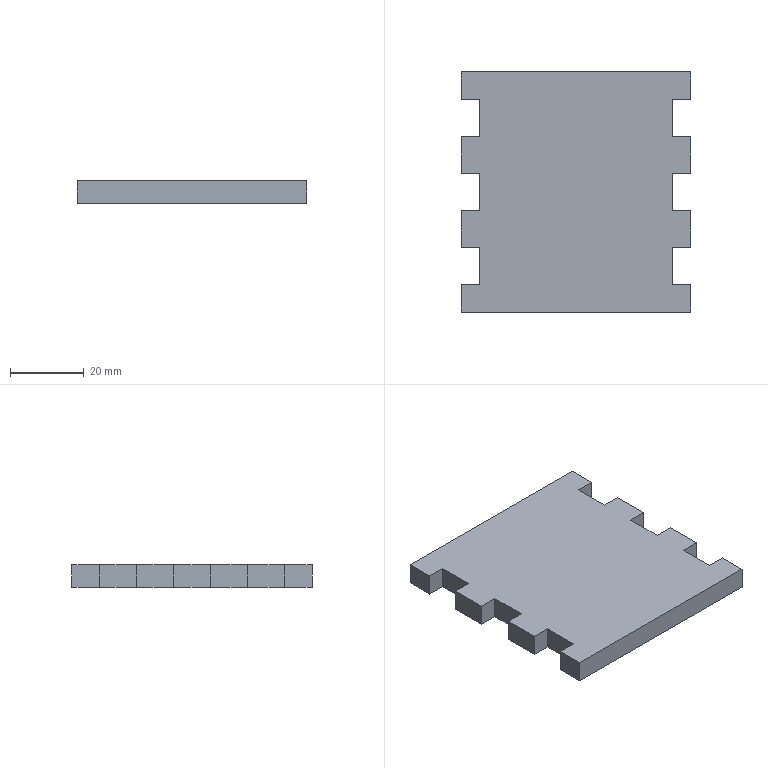Part | SolidWorks | features FlatPattern 1, SMBaseFlange 1, SheetMetal 1 | 1 solid | 30 faces | box 62 x 65 x 6 mm | volume 22380 mm3 | plane 30
STEP:
#1=CARTESIAN_POINT('',(31.,57.5,0.));
#2=VERTEX_POINT('',#1);
#3=CARTESIAN_POINT('',(31.,65.,0.));
#4=VERTEX_POINT('',#3);
#5=CARTESIAN_POINT('',(31.,65.,0.));
#6=DIRECTION('',(0.,1.,0.));
#7=VECTOR('',#6,1000.);
#8=LINE('',#5,#7);
#9=EDGE_CURVE('',#2,#4,#8,.T.);
#10=ORIENTED_EDGE('',*,*,#9,.T.);
#11=CARTESIAN_POINT('',(31.,65.,6.));
#12=VERTEX_POINT('',#11);
#13=CARTESIAN_POINT('',(31.,65.,6.));
#14=DIRECTION('',(0.,0.,-1.));
#15=VECTOR('',#14,1000.);
#16=LINE('',#13,#15);
#17=EDGE_CURVE('',#12,#4,#16,.T.);
#18=ORIENTED_EDGE('',*,*,#17,.F.);
#19=CARTESIAN_POINT('',(31.,57.5,6.));
#20=VERTEX_POINT('',#19);
#21=CARTESIAN_POINT('',(31.,65.,6.));
#22=DIRECTION('',(0.,1.,0.));
#23=VECTOR('',#22,1000.);
#24=LINE('',#21,#23);
#25=EDGE_CURVE('',#20,#12,#24,.T.);
#26=ORIENTED_EDGE('',*,*,#25,.F.);
#27=CARTESIAN_POINT('',(31.,57.5,6.));
#28=DIRECTION('',(0.,0.,-1.));
#29=VECTOR('',#28,1000.);
#30=LINE('',#27,#29);
#31=EDGE_CURVE('',#20,#2,#30,.T.);
#32=ORIENTED_EDGE('',*,*,#31,.T.);
#33=EDGE_LOOP('',(#10,#18,#26,#32));
#34=FACE_OUTER_BOUND('',#33,.T.);
#35=CARTESIAN_POINT('',(31.,65.,6.));
#36=DIRECTION('',(-1.,0.,0.));
#37=DIRECTION('',(0.,-1.,0.));
#38=AXIS2_PLACEMENT_3D('',#35,#36,#37);
#39=PLANE('',#38);
#40=ADVANCED_FACE('',(#34),#39,.F.);
#41=CARTESIAN_POINT('',(-31.,65.,0.));
#42=VERTEX_POINT('',#41);
#43=CARTESIAN_POINT('',(31.,65.,0.));
#44=DIRECTION('',(-1.,0.,0.));
#45=VECTOR('',#44,1000.);
#46=LINE('',#43,#45);
#47=EDGE_CURVE('',#4,#42,#46,.T.);
#48=ORIENTED_EDGE('',*,*,#47,.T.);
#49=CARTESIAN_POINT('',(-31.,65.,6.));
#50=VERTEX_POINT('',#49);
#51=CARTESIAN_POINT('',(-31.,65.,6.));
#52=DIRECTION('',(0.,0.,-1.));
#53=VECTOR('',#52,1000.);
#54=LINE('',#51,#53);
#55=EDGE_CURVE('',#50,#42,#54,.T.);
#56=ORIENTED_EDGE('',*,*,#55,.F.);
#57=CARTESIAN_POINT('',(31.,65.,6.));
#58=DIRECTION('',(-1.,0.,0.));
#59=VECTOR('',#58,1000.);
#60=LINE('',#57,#59);
#61=EDGE_CURVE('',#12,#50,#60,.T.);
#62=ORIENTED_EDGE('',*,*,#61,.F.);
#63=ORIENTED_EDGE('',*,*,#17,.T.);
#64=EDGE_LOOP('',(#48,#56,#62,#63));
#65=FACE_OUTER_BOUND('',#64,.T.);
#66=CARTESIAN_POINT('',(31.,65.,6.));
#67=DIRECTION('',(0.,-1.,0.));
#68=DIRECTION('',(1.,0.,0.));
#69=AXIS2_PLACEMENT_3D('',#66,#67,#68);
#70=PLANE('',#69);
#71=ADVANCED_FACE('',(#65),#70,.F.);
#72=CARTESIAN_POINT('',(-31.,57.5,0.));
#73=VERTEX_POINT('',#72);
#74=CARTESIAN_POINT('',(-31.,65.,0.));
#75=DIRECTION('',(0.,-1.,0.));
#76=VECTOR('',#75,1000.);
#77=LINE('',#74,#76);
#78=EDGE_CURVE('',#42,#73,#77,.T.);
#79=ORIENTED_EDGE('',*,*,#78,.T.);
#80=CARTESIAN_POINT('',(-31.,57.5,6.));
#81=VERTEX_POINT('',#80);
#82=CARTESIAN_POINT('',(-31.,57.5,6.));
#83=DIRECTION('',(0.,0.,-1.));
#84=VECTOR('',#83,1000.);
#85=LINE('',#82,#84);
#86=EDGE_CURVE('',#81,#73,#85,.T.);
#87=ORIENTED_EDGE('',*,*,#86,.F.);
#88=CARTESIAN_POINT('',(-31.,65.,6.));
#89=DIRECTION('',(0.,-1.,0.));
#90=VECTOR('',#89,1000.);
#91=LINE('',#88,#90);
#92=EDGE_CURVE('',#50,#81,#91,.T.);
#93=ORIENTED_EDGE('',*,*,#92,.F.);
#94=ORIENTED_EDGE('',*,*,#55,.T.);
#95=EDGE_LOOP('',(#79,#87,#93,#94));
#96=FACE_OUTER_BOUND('',#95,.T.);
#97=CARTESIAN_POINT('',(-31.,65.,6.));
#98=DIRECTION('',(1.,0.,0.));
#99=DIRECTION('',(0.,1.,0.));
#100=AXIS2_PLACEMENT_3D('',#97,#98,#99);
#101=PLANE('',#100);
#102=ADVANCED_FACE('',(#96),#101,.F.);
#103=CARTESIAN_POINT('',(-26.,57.5,0.));
#104=VERTEX_POINT('',#103);
#105=CARTESIAN_POINT('',(-31.,57.5,0.));
#106=DIRECTION('',(1.,0.,0.));
#107=VECTOR('',#106,1000.);
#108=LINE('',#105,#107);
#109=EDGE_CURVE('',#73,#104,#108,.T.);
#110=ORIENTED_EDGE('',*,*,#109,.T.);
#111=CARTESIAN_POINT('',(-26.,57.5,6.));
#112=VERTEX_POINT('',#111);
#113=CARTESIAN_POINT('',(-26.,57.5,6.));
#114=DIRECTION('',(0.,0.,-1.));
#115=VECTOR('',#114,1000.);
#116=LINE('',#113,#115);
#117=EDGE_CURVE('',#112,#104,#116,.T.);
#118=ORIENTED_EDGE('',*,*,#117,.F.);
#119=CARTESIAN_POINT('',(-31.,57.5,6.));
#120=DIRECTION('',(1.,0.,0.));
#121=VECTOR('',#120,1000.);
#122=LINE('',#119,#121);
#123=EDGE_CURVE('',#81,#112,#122,.T.);
#124=ORIENTED_EDGE('',*,*,#123,.F.);
#125=ORIENTED_EDGE('',*,*,#86,.T.);
#126=EDGE_LOOP('',(#110,#118,#124,#125));
#127=FACE_OUTER_BOUND('',#126,.T.);
#128=CARTESIAN_POINT('',(-31.,57.5,6.));
#129=DIRECTION('',(0.,1.,0.));
#130=DIRECTION('',(0.,0.,1.));
#131=AXIS2_PLACEMENT_3D('',#128,#129,#130);
#132=PLANE('',#131);
#133=ADVANCED_FACE('',(#127),#132,.F.);
#134=CARTESIAN_POINT('',(-26.,47.5,0.));
#135=VERTEX_POINT('',#134);
#136=CARTESIAN_POINT('',(-26.,57.5,0.));
#137=DIRECTION('',(0.,-1.,0.));
#138=VECTOR('',#137,1000.);
#139=LINE('',#136,#138);
#140=EDGE_CURVE('',#104,#135,#139,.T.);
#141=ORIENTED_EDGE('',*,*,#140,.T.);
#142=CARTESIAN_POINT('',(-26.,47.5,6.));
#143=VERTEX_POINT('',#142);
#144=CARTESIAN_POINT('',(-26.,47.5,6.));
#145=DIRECTION('',(0.,0.,-1.));
#146=VECTOR('',#145,1000.);
#147=LINE('',#144,#146);
#148=EDGE_CURVE('',#143,#135,#147,.T.);
#149=ORIENTED_EDGE('',*,*,#148,.F.);
#150=CARTESIAN_POINT('',(-26.,57.5,6.));
#151=DIRECTION('',(0.,-1.,0.));
#152=VECTOR('',#151,1000.);
#153=LINE('',#150,#152);
#154=EDGE_CURVE('',#112,#143,#153,.T.);
#155=ORIENTED_EDGE('',*,*,#154,.F.);
#156=ORIENTED_EDGE('',*,*,#117,.T.);
#157=EDGE_LOOP('',(#141,#149,#155,#156));
#158=FACE_OUTER_BOUND('',#157,.T.);
#159=CARTESIAN_POINT('',(-26.,57.5,6.));
#160=DIRECTION('',(1.,0.,0.));
#161=DIRECTION('',(0.,0.,-1.));
#162=AXIS2_PLACEMENT_3D('',#159,#160,#161);
#163=PLANE('',#162);
#164=ADVANCED_FACE('',(#158),#163,.F.);
#165=CARTESIAN_POINT('',(-31.,47.5,0.));
#166=VERTEX_POINT('',#165);
#167=CARTESIAN_POINT('',(-26.,47.5,0.));
#168=DIRECTION('',(-1.,0.,0.));
#169=VECTOR('',#168,1000.);
#170=LINE('',#167,#169);
#171=EDGE_CURVE('',#135,#166,#170,.T.);
#172=ORIENTED_EDGE('',*,*,#171,.T.);
#173=CARTESIAN_POINT('',(-31.,47.5,6.));
#174=VERTEX_POINT('',#173);
#175=CARTESIAN_POINT('',(-31.,47.5,6.));
#176=DIRECTION('',(0.,0.,-1.));
#177=VECTOR('',#176,1000.);
#178=LINE('',#175,#177);
#179=EDGE_CURVE('',#174,#166,#178,.T.);
#180=ORIENTED_EDGE('',*,*,#179,.F.);
#181=CARTESIAN_POINT('',(-26.,47.5,6.));
#182=DIRECTION('',(-1.,0.,0.));
#183=VECTOR('',#182,1000.);
#184=LINE('',#181,#183);
#185=EDGE_CURVE('',#143,#174,#184,.T.);
#186=ORIENTED_EDGE('',*,*,#185,.F.);
#187=ORIENTED_EDGE('',*,*,#148,.T.);
#188=EDGE_LOOP('',(#172,#180,#186,#187));
#189=FACE_OUTER_BOUND('',#188,.T.);
#190=CARTESIAN_POINT('',(-26.,47.5,6.));
#191=DIRECTION('',(0.,-1.,0.));
#192=DIRECTION('',(0.,0.,-1.));
#193=AXIS2_PLACEMENT_3D('',#190,#191,#192);
#194=PLANE('',#193);
#195=ADVANCED_FACE('',(#189),#194,.F.);
#196=CARTESIAN_POINT('',(-31.,37.5,0.));
#197=VERTEX_POINT('',#196);
#198=CARTESIAN_POINT('',(-31.,47.5,0.));
#199=DIRECTION('',(0.,-1.,0.));
#200=VECTOR('',#199,1000.);
#201=LINE('',#198,#200);
#202=EDGE_CURVE('',#166,#197,#201,.T.);
#203=ORIENTED_EDGE('',*,*,#202,.T.);
#204=CARTESIAN_POINT('',(-31.,37.5,6.));
#205=VERTEX_POINT('',#204);
#206=CARTESIAN_POINT('',(-31.,37.5,6.));
#207=DIRECTION('',(0.,0.,-1.));
#208=VECTOR('',#207,1000.);
#209=LINE('',#206,#208);
#210=EDGE_CURVE('',#205,#197,#209,.T.);
#211=ORIENTED_EDGE('',*,*,#210,.F.);
#212=CARTESIAN_POINT('',(-31.,47.5,6.));
#213=DIRECTION('',(0.,-1.,0.));
#214=VECTOR('',#213,1000.);
#215=LINE('',#212,#214);
#216=EDGE_CURVE('',#174,#205,#215,.T.);
#217=ORIENTED_EDGE('',*,*,#216,.F.);
#218=ORIENTED_EDGE('',*,*,#179,.T.);
#219=EDGE_LOOP('',(#203,#211,#217,#218));
#220=FACE_OUTER_BOUND('',#219,.T.);
#221=CARTESIAN_POINT('',(-31.,47.5,6.));
#222=DIRECTION('',(1.,0.,0.));
#223=DIRECTION('',(0.,0.,-1.));
#224=AXIS2_PLACEMENT_3D('',#221,#222,#223);
#225=PLANE('',#224);
#226=ADVANCED_FACE('',(#220),#225,.F.);
#227=CARTESIAN_POINT('',(-26.,37.5,0.));
#228=VERTEX_POINT('',#227);
#229=CARTESIAN_POINT('',(-31.,37.5,0.));
#230=DIRECTION('',(1.,0.,0.));
#231=VECTOR('',#230,1000.);
#232=LINE('',#229,#231);
#233=EDGE_CURVE('',#197,#228,#232,.T.);
#234=ORIENTED_EDGE('',*,*,#233,.T.);
#235=CARTESIAN_POINT('',(-26.,37.5,6.));
#236=VERTEX_POINT('',#235);
#237=CARTESIAN_POINT('',(-26.,37.5,6.));
#238=DIRECTION('',(0.,0.,-1.));
#239=VECTOR('',#238,1000.);
#240=LINE('',#237,#239);
#241=EDGE_CURVE('',#236,#228,#240,.T.);
#242=ORIENTED_EDGE('',*,*,#241,.F.);
#243=CARTESIAN_POINT('',(-31.,37.5,6.));
#244=DIRECTION('',(1.,0.,0.));
#245=VECTOR('',#244,1000.);
#246=LINE('',#243,#245);
#247=EDGE_CURVE('',#205,#236,#246,.T.);
#248=ORIENTED_EDGE('',*,*,#247,.F.);
#249=ORIENTED_EDGE('',*,*,#210,.T.);
#250=EDGE_LOOP('',(#234,#242,#248,#249));
#251=FACE_OUTER_BOUND('',#250,.T.);
#252=CARTESIAN_POINT('',(-31.,37.5,6.));
#253=DIRECTION('',(0.,1.,0.));
#254=DIRECTION('',(0.,0.,1.));
#255=AXIS2_PLACEMENT_3D('',#252,#253,#254);
#256=PLANE('',#255);
#257=ADVANCED_FACE('',(#251),#256,.F.);
#258=CARTESIAN_POINT('',(-26.,27.5,0.));
#259=VERTEX_POINT('',#258);
#260=CARTESIAN_POINT('',(-26.,37.5,0.));
#261=DIRECTION('',(0.,-1.,0.));
#262=VECTOR('',#261,1000.);
#263=LINE('',#260,#262);
#264=EDGE_CURVE('',#228,#259,#263,.T.);
#265=ORIENTED_EDGE('',*,*,#264,.T.);
#266=CARTESIAN_POINT('',(-26.,27.5,6.));
#267=VERTEX_POINT('',#266);
#268=CARTESIAN_POINT('',(-26.,27.5,6.));
#269=DIRECTION('',(0.,0.,-1.));
#270=VECTOR('',#269,1000.);
#271=LINE('',#268,#270);
#272=EDGE_CURVE('',#267,#259,#271,.T.);
#273=ORIENTED_EDGE('',*,*,#272,.F.);
#274=CARTESIAN_POINT('',(-26.,37.5,6.));
#275=DIRECTION('',(0.,-1.,0.));
#276=VECTOR('',#275,1000.);
#277=LINE('',#274,#276);
#278=EDGE_CURVE('',#236,#267,#277,.T.);
#279=ORIENTED_EDGE('',*,*,#278,.F.);
#280=ORIENTED_EDGE('',*,*,#241,.T.);
#281=EDGE_LOOP('',(#265,#273,#279,#280));
#282=FACE_OUTER_BOUND('',#281,.T.);
#283=CARTESIAN_POINT('',(-26.,37.5,6.));
#284=DIRECTION('',(1.,0.,0.));
#285=DIRECTION('',(0.,0.,-1.));
#286=AXIS2_PLACEMENT_3D('',#283,#284,#285);
#287=PLANE('',#286);
#288=ADVANCED_FACE('',(#282),#287,.F.);
#289=CARTESIAN_POINT('',(-31.,27.5,0.));
#290=VERTEX_POINT('',#289);
#291=CARTESIAN_POINT('',(-26.,27.5,0.));
#292=DIRECTION('',(-1.,0.,0.));
#293=VECTOR('',#292,1000.);
#294=LINE('',#291,#293);
#295=EDGE_CURVE('',#259,#290,#294,.T.);
#296=ORIENTED_EDGE('',*,*,#295,.T.);
#297=CARTESIAN_POINT('',(-31.,27.5,6.));
#298=VERTEX_POINT('',#297);
#299=CARTESIAN_POINT('',(-31.,27.5,6.));
#300=DIRECTION('',(0.,0.,-1.));
#301=VECTOR('',#300,1000.);
#302=LINE('',#299,#301);
#303=EDGE_CURVE('',#298,#290,#302,.T.);
#304=ORIENTED_EDGE('',*,*,#303,.F.);
#305=CARTESIAN_POINT('',(-26.,27.5,6.));
#306=DIRECTION('',(-1.,0.,0.));
#307=VECTOR('',#306,1000.);
#308=LINE('',#305,#307);
#309=EDGE_CURVE('',#267,#298,#308,.T.);
#310=ORIENTED_EDGE('',*,*,#309,.F.);
#311=ORIENTED_EDGE('',*,*,#272,.T.);
#312=EDGE_LOOP('',(#296,#304,#310,#311));
#313=FACE_OUTER_BOUND('',#312,.T.);
#314=CARTESIAN_POINT('',(-26.,27.5,6.));
#315=DIRECTION('',(0.,-1.,0.));
#316=DIRECTION('',(0.,0.,-1.));
#317=AXIS2_PLACEMENT_3D('',#314,#315,#316);
#318=PLANE('',#317);
#319=ADVANCED_FACE('',(#313),#318,.F.);
#320=CARTESIAN_POINT('',(-31.,17.5,0.));
#321=VERTEX_POINT('',#320);
#322=CARTESIAN_POINT('',(-31.,27.5,0.));
#323=DIRECTION('',(0.,-1.,0.));
#324=VECTOR('',#323,1000.);
#325=LINE('',#322,#324);
#326=EDGE_CURVE('',#290,#321,#325,.T.);
#327=ORIENTED_EDGE('',*,*,#326,.T.);
#328=CARTESIAN_POINT('',(-31.,17.5,6.));
#329=VERTEX_POINT('',#328);
#330=CARTESIAN_POINT('',(-31.,17.5,6.));
#331=DIRECTION('',(0.,0.,-1.));
#332=VECTOR('',#331,1000.);
#333=LINE('',#330,#332);
#334=EDGE_CURVE('',#329,#321,#333,.T.);
#335=ORIENTED_EDGE('',*,*,#334,.F.);
#336=CARTESIAN_POINT('',(-31.,27.5,6.));
#337=DIRECTION('',(0.,-1.,0.));
#338=VECTOR('',#337,1000.);
#339=LINE('',#336,#338);
#340=EDGE_CURVE('',#298,#329,#339,.T.);
#341=ORIENTED_EDGE('',*,*,#340,.F.);
#342=ORIENTED_EDGE('',*,*,#303,.T.);
#343=EDGE_LOOP('',(#327,#335,#341,#342));
#344=FACE_OUTER_BOUND('',#343,.T.);
#345=CARTESIAN_POINT('',(-31.,27.5,6.));
#346=DIRECTION('',(1.,0.,0.));
#347=DIRECTION('',(0.,0.,-1.));
#348=AXIS2_PLACEMENT_3D('',#345,#346,#347);
#349=PLANE('',#348);
#350=ADVANCED_FACE('',(#344),#349,.F.);
#351=CARTESIAN_POINT('',(-26.,17.5,0.));
#352=VERTEX_POINT('',#351);
#353=CARTESIAN_POINT('',(-31.,17.5,0.));
#354=DIRECTION('',(1.,0.,0.));
#355=VECTOR('',#354,1000.);
#356=LINE('',#353,#355);
#357=EDGE_CURVE('',#321,#352,#356,.T.);
#358=ORIENTED_EDGE('',*,*,#357,.T.);
#359=CARTESIAN_POINT('',(-26.,17.5,6.));
#360=VERTEX_POINT('',#359);
#361=CARTESIAN_POINT('',(-26.,17.5,6.));
#362=DIRECTION('',(0.,0.,-1.));
#363=VECTOR('',#362,1000.);
#364=LINE('',#361,#363);
#365=EDGE_CURVE('',#360,#352,#364,.T.);
#366=ORIENTED_EDGE('',*,*,#365,.F.);
#367=CARTESIAN_POINT('',(-31.,17.5,6.));
#368=DIRECTION('',(1.,0.,0.));
#369=VECTOR('',#368,1000.);
#370=LINE('',#367,#369);
#371=EDGE_CURVE('',#329,#360,#370,.T.);
#372=ORIENTED_EDGE('',*,*,#371,.F.);
#373=ORIENTED_EDGE('',*,*,#334,.T.);
#374=EDGE_LOOP('',(#358,#366,#372,#373));
#375=FACE_OUTER_BOUND('',#374,.T.);
#376=CARTESIAN_POINT('',(-31.,17.5,6.));
#377=DIRECTION('',(0.,1.,0.));
#378=DIRECTION('',(0.,0.,1.));
#379=AXIS2_PLACEMENT_3D('',#376,#377,#378);
#380=PLANE('',#379);
#381=ADVANCED_FACE('',(#375),#380,.F.);
#382=CARTESIAN_POINT('',(-26.,7.5,0.));
#383=VERTEX_POINT('',#382);
#384=CARTESIAN_POINT('',(-26.,17.5,0.));
#385=DIRECTION('',(0.,-1.,0.));
#386=VECTOR('',#385,1000.);
#387=LINE('',#384,#386);
#388=EDGE_CURVE('',#352,#383,#387,.T.);
#389=ORIENTED_EDGE('',*,*,#388,.T.);
#390=CARTESIAN_POINT('',(-26.,7.5,6.));
#391=VERTEX_POINT('',#390);
#392=CARTESIAN_POINT('',(-26.,7.5,6.));
#393=DIRECTION('',(0.,0.,-1.));
#394=VECTOR('',#393,1000.);
#395=LINE('',#392,#394);
#396=EDGE_CURVE('',#391,#383,#395,.T.);
#397=ORIENTED_EDGE('',*,*,#396,.F.);
#398=CARTESIAN_POINT('',(-26.,17.5,6.));
#399=DIRECTION('',(0.,-1.,0.));
#400=VECTOR('',#399,1000.);
#401=LINE('',#398,#400);
#402=EDGE_CURVE('',#360,#391,#401,.T.);
#403=ORIENTED_EDGE('',*,*,#402,.F.);
#404=ORIENTED_EDGE('',*,*,#365,.T.);
#405=EDGE_LOOP('',(#389,#397,#403,#404));
#406=FACE_OUTER_BOUND('',#405,.T.);
#407=CARTESIAN_POINT('',(-26.,17.5,6.));
#408=DIRECTION('',(1.,0.,0.));
#409=DIRECTION('',(0.,0.,-1.));
#410=AXIS2_PLACEMENT_3D('',#407,#408,#409);
#411=PLANE('',#410);
#412=ADVANCED_FACE('',(#406),#411,.F.);
#413=CARTESIAN_POINT('',(-31.,7.5,0.));
#414=VERTEX_POINT('',#413);
#415=CARTESIAN_POINT('',(-26.,7.5,0.));
#416=DIRECTION('',(-1.,0.,0.));
#417=VECTOR('',#416,1000.);
#418=LINE('',#415,#417);
#419=EDGE_CURVE('',#383,#414,#418,.T.);
#420=ORIENTED_EDGE('',*,*,#419,.T.);
#421=CARTESIAN_POINT('',(-31.,7.5,6.));
#422=VERTEX_POINT('',#421);
#423=CARTESIAN_POINT('',(-31.,7.5,6.));
#424=DIRECTION('',(0.,0.,-1.));
#425=VECTOR('',#424,1000.);
#426=LINE('',#423,#425);
#427=EDGE_CURVE('',#422,#414,#426,.T.);
#428=ORIENTED_EDGE('',*,*,#427,.F.);
#429=CARTESIAN_POINT('',(-26.,7.5,6.));
#430=DIRECTION('',(-1.,0.,0.));
#431=VECTOR('',#430,1000.);
#432=LINE('',#429,#431);
#433=EDGE_CURVE('',#391,#422,#432,.T.);
#434=ORIENTED_EDGE('',*,*,#433,.F.);
#435=ORIENTED_EDGE('',*,*,#396,.T.);
#436=EDGE_LOOP('',(#420,#428,#434,#435));
#437=FACE_OUTER_BOUND('',#436,.T.);
#438=CARTESIAN_POINT('',(-26.,7.5,6.));
#439=DIRECTION('',(0.,-1.,0.));
#440=DIRECTION('',(0.,0.,-1.));
#441=AXIS2_PLACEMENT_3D('',#438,#439,#440);
#442=PLANE('',#441);
#443=ADVANCED_FACE('',(#437),#442,.F.);
#444=CARTESIAN_POINT('',(-31.,0.,0.));
#445=VERTEX_POINT('',#444);
#446=CARTESIAN_POINT('',(-31.,7.5,0.));
#447=DIRECTION('',(0.,-1.,0.));
#448=VECTOR('',#447,1000.);
#449=LINE('',#446,#448);
#450=EDGE_CURVE('',#414,#445,#449,.T.);
#451=ORIENTED_EDGE('',*,*,#450,.T.);
#452=CARTESIAN_POINT('',(-31.,0.,6.));
#453=VERTEX_POINT('',#452);
#454=CARTESIAN_POINT('',(-31.,0.,6.));
#455=DIRECTION('',(0.,0.,-1.));
#456=VECTOR('',#455,1000.);
#457=LINE('',#454,#456);
#458=EDGE_CURVE('',#453,#445,#457,.T.);
#459=ORIENTED_EDGE('',*,*,#458,.F.);
#460=CARTESIAN_POINT('',(-31.,7.5,6.));
#461=DIRECTION('',(0.,-1.,0.));
#462=VECTOR('',#461,1000.);
#463=LINE('',#460,#462);
#464=EDGE_CURVE('',#422,#453,#463,.T.);
#465=ORIENTED_EDGE('',*,*,#464,.F.);
#466=ORIENTED_EDGE('',*,*,#427,.T.);
#467=EDGE_LOOP('',(#451,#459,#465,#466));
#468=FACE_OUTER_BOUND('',#467,.T.);
#469=CARTESIAN_POINT('',(-31.,7.5,6.));
#470=DIRECTION('',(1.,0.,0.));
#471=DIRECTION('',(0.,0.,-1.));
#472=AXIS2_PLACEMENT_3D('',#469,#470,#471);
#473=PLANE('',#472);
#474=ADVANCED_FACE('',(#468),#473,.F.);
#475=CARTESIAN_POINT('',(31.,0.,0.));
#476=VERTEX_POINT('',#475);
#477=CARTESIAN_POINT('',(-31.,0.,0.));
#478=DIRECTION('',(1.,0.,0.));
#479=VECTOR('',#478,1000.);
#480=LINE('',#477,#479);
#481=EDGE_CURVE('',#445,#476,#480,.T.);
#482=ORIENTED_EDGE('',*,*,#481,.T.);
#483=CARTESIAN_POINT('',(31.,0.,6.));
#484=VERTEX_POINT('',#483);
#485=CARTESIAN_POINT('',(31.,0.,6.));
#486=DIRECTION('',(0.,0.,-1.));
#487=VECTOR('',#486,1000.);
#488=LINE('',#485,#487);
#489=EDGE_CURVE('',#484,#476,#488,.T.);
#490=ORIENTED_EDGE('',*,*,#489,.F.);
#491=CARTESIAN_POINT('',(-31.,0.,6.));
#492=DIRECTION('',(1.,0.,0.));
#493=VECTOR('',#492,1000.);
#494=LINE('',#491,#493);
#495=EDGE_CURVE('',#453,#484,#494,.T.);
#496=ORIENTED_EDGE('',*,*,#495,.F.);
#497=ORIENTED_EDGE('',*,*,#458,.T.);
#498=EDGE_LOOP('',(#482,#490,#496,#497));
#499=FACE_OUTER_BOUND('',#498,.T.);
#500=CARTESIAN_POINT('',(-31.,0.,6.));
#501=DIRECTION('',(0.,1.,0.));
#502=DIRECTION('',(0.,0.,1.));
#503=AXIS2_PLACEMENT_3D('',#500,#501,#502);
#504=PLANE('',#503);
#505=ADVANCED_FACE('',(#499),#504,.F.);
#506=CARTESIAN_POINT('',(31.,7.5,0.));
#507=VERTEX_POINT('',#506);
#508=CARTESIAN_POINT('',(31.,7.5,0.));
#509=DIRECTION('',(0.,1.,0.));
#510=VECTOR('',#509,1000.);
#511=LINE('',#508,#510);
#512=EDGE_CURVE('',#476,#507,#511,.T.);
#513=ORIENTED_EDGE('',*,*,#512,.T.);
#514=CARTESIAN_POINT('',(31.,7.5,6.));
#515=VERTEX_POINT('',#514);
#516=CARTESIAN_POINT('',(31.,7.5,6.));
#517=DIRECTION('',(0.,0.,-1.));
#518=VECTOR('',#517,1000.);
#519=LINE('',#516,#518);
#520=EDGE_CURVE('',#515,#507,#519,.T.);
#521=ORIENTED_EDGE('',*,*,#520,.F.);
#522=CARTESIAN_POINT('',(31.,7.5,6.));
#523=DIRECTION('',(0.,1.,0.));
#524=VECTOR('',#523,1000.);
#525=LINE('',#522,#524);
#526=EDGE_CURVE('',#484,#515,#525,.T.);
#527=ORIENTED_EDGE('',*,*,#526,.F.);
#528=ORIENTED_EDGE('',*,*,#489,.T.);
#529=EDGE_LOOP('',(#513,#521,#527,#528));
#530=FACE_OUTER_BOUND('',#529,.T.);
#531=CARTESIAN_POINT('',(31.,7.5,6.));
#532=DIRECTION('',(-1.,0.,0.));
#533=DIRECTION('',(0.,-1.,0.));
#534=AXIS2_PLACEMENT_3D('',#531,#532,#533);
#535=PLANE('',#534);
#536=ADVANCED_FACE('',(#530),#535,.F.);
#537=CARTESIAN_POINT('',(26.,7.5,0.));
#538=VERTEX_POINT('',#537);
#539=CARTESIAN_POINT('',(26.,7.5,0.));
#540=DIRECTION('',(-1.,0.,0.));
#541=VECTOR('',#540,1000.);
#542=LINE('',#539,#541);
#543=EDGE_CURVE('',#507,#538,#542,.T.);
#544=ORIENTED_EDGE('',*,*,#543,.T.);
#545=CARTESIAN_POINT('',(26.,7.5,6.));
#546=VERTEX_POINT('',#545);
#547=CARTESIAN_POINT('',(26.,7.5,6.));
#548=DIRECTION('',(0.,0.,-1.));
#549=VECTOR('',#548,1000.);
#550=LINE('',#547,#549);
#551=EDGE_CURVE('',#546,#538,#550,.T.);
#552=ORIENTED_EDGE('',*,*,#551,.F.);
#553=CARTESIAN_POINT('',(26.,7.5,6.));
#554=DIRECTION('',(-1.,0.,0.));
#555=VECTOR('',#554,1000.);
#556=LINE('',#553,#555);
#557=EDGE_CURVE('',#515,#546,#556,.T.);
#558=ORIENTED_EDGE('',*,*,#557,.F.);
#559=ORIENTED_EDGE('',*,*,#520,.T.);
#560=EDGE_LOOP('',(#544,#552,#558,#559));
#561=FACE_OUTER_BOUND('',#560,.T.);
#562=CARTESIAN_POINT('',(26.,7.5,6.));
#563=DIRECTION('',(0.,-1.,0.));
#564=DIRECTION('',(0.,0.,-1.));
#565=AXIS2_PLACEMENT_3D('',#562,#563,#564);
#566=PLANE('',#565);
#567=ADVANCED_FACE('',(#561),#566,.F.);
#568=CARTESIAN_POINT('',(26.,17.5,0.));
#569=VERTEX_POINT('',#568);
#570=CARTESIAN_POINT('',(26.,17.5,0.));
#571=DIRECTION('',(0.,1.,0.));
#572=VECTOR('',#571,1000.);
#573=LINE('',#570,#572);
#574=EDGE_CURVE('',#538,#569,#573,.T.);
#575=ORIENTED_EDGE('',*,*,#574,.T.);
#576=CARTESIAN_POINT('',(26.,17.5,6.));
#577=VERTEX_POINT('',#576);
#578=CARTESIAN_POINT('',(26.,17.5,6.));
#579=DIRECTION('',(0.,0.,-1.));
#580=VECTOR('',#579,1000.);
#581=LINE('',#578,#580);
#582=EDGE_CURVE('',#577,#569,#581,.T.);
#583=ORIENTED_EDGE('',*,*,#582,.F.);
#584=CARTESIAN_POINT('',(26.,17.5,6.));
#585=DIRECTION('',(0.,1.,0.));
#586=VECTOR('',#585,1000.);
#587=LINE('',#584,#586);
#588=EDGE_CURVE('',#546,#577,#587,.T.);
#589=ORIENTED_EDGE('',*,*,#588,.F.);
#590=ORIENTED_EDGE('',*,*,#551,.T.);
#591=EDGE_LOOP('',(#575,#583,#589,#590));
#592=FACE_OUTER_BOUND('',#591,.T.);
#593=CARTESIAN_POINT('',(26.,17.5,6.));
#594=DIRECTION('',(-1.,0.,0.));
#595=DIRECTION('',(0.,0.,1.));
#596=AXIS2_PLACEMENT_3D('',#593,#594,#595);
#597=PLANE('',#596);
#598=ADVANCED_FACE('',(#592),#597,.F.);
#599=CARTESIAN_POINT('',(31.,17.5,0.));
#600=VERTEX_POINT('',#599);
#601=CARTESIAN_POINT('',(31.,17.5,0.));
#602=DIRECTION('',(1.,0.,0.));
#603=VECTOR('',#602,1000.);
#604=LINE('',#601,#603);
#605=EDGE_CURVE('',#569,#600,#604,.T.);
#606=ORIENTED_EDGE('',*,*,#605,.T.);
#607=CARTESIAN_POINT('',(31.,17.5,6.));
#608=VERTEX_POINT('',#607);
#609=CARTESIAN_POINT('',(31.,17.5,6.));
#610=DIRECTION('',(0.,0.,-1.));
#611=VECTOR('',#610,1000.);
#612=LINE('',#609,#611);
#613=EDGE_CURVE('',#608,#600,#612,.T.);
#614=ORIENTED_EDGE('',*,*,#613,.F.);
#615=CARTESIAN_POINT('',(31.,17.5,6.));
#616=DIRECTION('',(1.,0.,0.));
#617=VECTOR('',#616,1000.);
#618=LINE('',#615,#617);
#619=EDGE_CURVE('',#577,#608,#618,.T.);
#620=ORIENTED_EDGE('',*,*,#619,.F.);
#621=ORIENTED_EDGE('',*,*,#582,.T.);
#622=EDGE_LOOP('',(#606,#614,#620,#621));
#623=FACE_OUTER_BOUND('',#622,.T.);
#624=CARTESIAN_POINT('',(31.,17.5,6.));
#625=DIRECTION('',(0.,1.,0.));
#626=DIRECTION('',(0.,0.,1.));
#627=AXIS2_PLACEMENT_3D('',#624,#625,#626);
#628=PLANE('',#627);
#629=ADVANCED_FACE('',(#623),#628,.F.);
#630=CARTESIAN_POINT('',(31.,27.5,0.));
#631=VERTEX_POINT('',#630);
#632=CARTESIAN_POINT('',(31.,27.5,0.));
#633=DIRECTION('',(0.,1.,0.));
#634=VECTOR('',#633,1000.);
#635=LINE('',#632,#634);
#636=EDGE_CURVE('',#600,#631,#635,.T.);
#637=ORIENTED_EDGE('',*,*,#636,.T.);
#638=CARTESIAN_POINT('',(31.,27.5,6.));
#639=VERTEX_POINT('',#638);
#640=CARTESIAN_POINT('',(31.,27.5,6.));
#641=DIRECTION('',(0.,0.,-1.));
#642=VECTOR('',#641,1000.);
#643=LINE('',#640,#642);
#644=EDGE_CURVE('',#639,#631,#643,.T.);
#645=ORIENTED_EDGE('',*,*,#644,.F.);
#646=CARTESIAN_POINT('',(31.,27.5,6.));
#647=DIRECTION('',(0.,1.,0.));
#648=VECTOR('',#647,1000.);
#649=LINE('',#646,#648);
#650=EDGE_CURVE('',#608,#639,#649,.T.);
#651=ORIENTED_EDGE('',*,*,#650,.F.);
#652=ORIENTED_EDGE('',*,*,#613,.T.);
#653=EDGE_LOOP('',(#637,#645,#651,#652));
#654=FACE_OUTER_BOUND('',#653,.T.);
#655=CARTESIAN_POINT('',(31.,27.5,6.));
#656=DIRECTION('',(-1.,0.,0.));
#657=DIRECTION('',(0.,0.,1.));
#658=AXIS2_PLACEMENT_3D('',#655,#656,#657);
#659=PLANE('',#658);
#660=ADVANCED_FACE('',(#654),#659,.F.);
#661=CARTESIAN_POINT('',(26.,27.5,0.));
#662=VERTEX_POINT('',#661);
#663=CARTESIAN_POINT('',(26.,27.5,0.));
#664=DIRECTION('',(-1.,0.,0.));
#665=VECTOR('',#664,1000.);
#666=LINE('',#663,#665);
#667=EDGE_CURVE('',#631,#662,#666,.T.);
#668=ORIENTED_EDGE('',*,*,#667,.T.);
#669=CARTESIAN_POINT('',(26.,27.5,6.));
#670=VERTEX_POINT('',#669);
#671=CARTESIAN_POINT('',(26.,27.5,6.));
#672=DIRECTION('',(0.,0.,-1.));
#673=VECTOR('',#672,1000.);
#674=LINE('',#671,#673);
#675=EDGE_CURVE('',#670,#662,#674,.T.);
#676=ORIENTED_EDGE('',*,*,#675,.F.);
#677=CARTESIAN_POINT('',(26.,27.5,6.));
#678=DIRECTION('',(-1.,0.,0.));
#679=VECTOR('',#678,1000.);
#680=LINE('',#677,#679);
#681=EDGE_CURVE('',#639,#670,#680,.T.);
#682=ORIENTED_EDGE('',*,*,#681,.F.);
#683=ORIENTED_EDGE('',*,*,#644,.T.);
#684=EDGE_LOOP('',(#668,#676,#682,#683));
#685=FACE_OUTER_BOUND('',#684,.T.);
#686=CARTESIAN_POINT('',(26.,27.5,6.));
#687=DIRECTION('',(0.,-1.,0.));
#688=DIRECTION('',(0.,0.,-1.));
#689=AXIS2_PLACEMENT_3D('',#686,#687,#688);
#690=PLANE('',#689);
#691=ADVANCED_FACE('',(#685),#690,.F.);
#692=CARTESIAN_POINT('',(26.,37.5,0.));
#693=VERTEX_POINT('',#692);
#694=CARTESIAN_POINT('',(26.,37.5,0.));
#695=DIRECTION('',(0.,1.,0.));
#696=VECTOR('',#695,1000.);
#697=LINE('',#694,#696);
#698=EDGE_CURVE('',#662,#693,#697,.T.);
#699=ORIENTED_EDGE('',*,*,#698,.T.);
#700=CARTESIAN_POINT('',(26.,37.5,6.));
#701=VERTEX_POINT('',#700);
#702=CARTESIAN_POINT('',(26.,37.5,6.));
#703=DIRECTION('',(0.,0.,-1.));
#704=VECTOR('',#703,1000.);
#705=LINE('',#702,#704);
#706=EDGE_CURVE('',#701,#693,#705,.T.);
#707=ORIENTED_EDGE('',*,*,#706,.F.);
#708=CARTESIAN_POINT('',(26.,37.5,6.));
#709=DIRECTION('',(0.,1.,0.));
#710=VECTOR('',#709,1000.);
#711=LINE('',#708,#710);
#712=EDGE_CURVE('',#670,#701,#711,.T.);
#713=ORIENTED_EDGE('',*,*,#712,.F.);
#714=ORIENTED_EDGE('',*,*,#675,.T.);
#715=EDGE_LOOP('',(#699,#707,#713,#714));
#716=FACE_OUTER_BOUND('',#715,.T.);
#717=CARTESIAN_POINT('',(26.,37.5,6.));
#718=DIRECTION('',(-1.,0.,0.));
#719=DIRECTION('',(0.,0.,1.));
#720=AXIS2_PLACEMENT_3D('',#717,#718,#719);
#721=PLANE('',#720);
#722=ADVANCED_FACE('',(#716),#721,.F.);
#723=CARTESIAN_POINT('',(31.,37.5,0.));
#724=VERTEX_POINT('',#723);
#725=CARTESIAN_POINT('',(31.,37.5,0.));
#726=DIRECTION('',(1.,0.,0.));
#727=VECTOR('',#726,1000.);
#728=LINE('',#725,#727);
#729=EDGE_CURVE('',#693,#724,#728,.T.);
#730=ORIENTED_EDGE('',*,*,#729,.T.);
#731=CARTESIAN_POINT('',(31.,37.5,6.));
#732=VERTEX_POINT('',#731);
#733=CARTESIAN_POINT('',(31.,37.5,6.));
#734=DIRECTION('',(0.,0.,-1.));
#735=VECTOR('',#734,1000.);
#736=LINE('',#733,#735);
#737=EDGE_CURVE('',#732,#724,#736,.T.);
#738=ORIENTED_EDGE('',*,*,#737,.F.);
#739=CARTESIAN_POINT('',(31.,37.5,6.));
#740=DIRECTION('',(1.,0.,0.));
#741=VECTOR('',#740,1000.);
#742=LINE('',#739,#741);
#743=EDGE_CURVE('',#701,#732,#742,.T.);
#744=ORIENTED_EDGE('',*,*,#743,.F.);
#745=ORIENTED_EDGE('',*,*,#706,.T.);
#746=EDGE_LOOP('',(#730,#738,#744,#745));
#747=FACE_OUTER_BOUND('',#746,.T.);
#748=CARTESIAN_POINT('',(31.,37.5,6.));
#749=DIRECTION('',(0.,1.,0.));
#750=DIRECTION('',(0.,0.,1.));
#751=AXIS2_PLACEMENT_3D('',#748,#749,#750);
#752=PLANE('',#751);
#753=ADVANCED_FACE('',(#747),#752,.F.);
#754=CARTESIAN_POINT('',(31.,47.5,0.));
#755=VERTEX_POINT('',#754);
#756=CARTESIAN_POINT('',(31.,47.5,0.));
#757=DIRECTION('',(0.,1.,0.));
#758=VECTOR('',#757,1000.);
#759=LINE('',#756,#758);
#760=EDGE_CURVE('',#724,#755,#759,.T.);
#761=ORIENTED_EDGE('',*,*,#760,.T.);
#762=CARTESIAN_POINT('',(31.,47.5,6.));
#763=VERTEX_POINT('',#762);
#764=CARTESIAN_POINT('',(31.,47.5,6.));
#765=DIRECTION('',(0.,0.,-1.));
#766=VECTOR('',#765,1000.);
#767=LINE('',#764,#766);
#768=EDGE_CURVE('',#763,#755,#767,.T.);
#769=ORIENTED_EDGE('',*,*,#768,.F.);
#770=CARTESIAN_POINT('',(31.,47.5,6.));
#771=DIRECTION('',(0.,1.,0.));
#772=VECTOR('',#771,1000.);
#773=LINE('',#770,#772);
#774=EDGE_CURVE('',#732,#763,#773,.T.);
#775=ORIENTED_EDGE('',*,*,#774,.F.);
#776=ORIENTED_EDGE('',*,*,#737,.T.);
#777=EDGE_LOOP('',(#761,#769,#775,#776));
#778=FACE_OUTER_BOUND('',#777,.T.);
#779=CARTESIAN_POINT('',(31.,47.5,6.));
#780=DIRECTION('',(-1.,0.,0.));
#781=DIRECTION('',(0.,0.,1.));
#782=AXIS2_PLACEMENT_3D('',#779,#780,#781);
#783=PLANE('',#782);
#784=ADVANCED_FACE('',(#778),#783,.F.);
#785=CARTESIAN_POINT('',(26.,47.5,0.));
#786=VERTEX_POINT('',#785);
#787=CARTESIAN_POINT('',(26.,47.5,0.));
#788=DIRECTION('',(-1.,0.,0.));
#789=VECTOR('',#788,1000.);
#790=LINE('',#787,#789);
#791=EDGE_CURVE('',#755,#786,#790,.T.);
#792=ORIENTED_EDGE('',*,*,#791,.T.);
#793=CARTESIAN_POINT('',(26.,47.5,6.));
#794=VERTEX_POINT('',#793);
#795=CARTESIAN_POINT('',(26.,47.5,6.));
#796=DIRECTION('',(0.,0.,-1.));
#797=VECTOR('',#796,1000.);
#798=LINE('',#795,#797);
#799=EDGE_CURVE('',#794,#786,#798,.T.);
#800=ORIENTED_EDGE('',*,*,#799,.F.);
#801=CARTESIAN_POINT('',(26.,47.5,6.));
#802=DIRECTION('',(-1.,0.,0.));
#803=VECTOR('',#802,1000.);
#804=LINE('',#801,#803);
#805=EDGE_CURVE('',#763,#794,#804,.T.);
#806=ORIENTED_EDGE('',*,*,#805,.F.);
#807=ORIENTED_EDGE('',*,*,#768,.T.);
#808=EDGE_LOOP('',(#792,#800,#806,#807));
#809=FACE_OUTER_BOUND('',#808,.T.);
#810=CARTESIAN_POINT('',(26.,47.5,6.));
#811=DIRECTION('',(0.,-1.,0.));
#812=DIRECTION('',(0.,0.,-1.));
#813=AXIS2_PLACEMENT_3D('',#810,#811,#812);
#814=PLANE('',#813);
#815=ADVANCED_FACE('',(#809),#814,.F.);
#816=CARTESIAN_POINT('',(26.,57.5,0.));
#817=VERTEX_POINT('',#816);
#818=CARTESIAN_POINT('',(26.,57.5,0.));
#819=DIRECTION('',(0.,1.,0.));
#820=VECTOR('',#819,1000.);
#821=LINE('',#818,#820);
#822=EDGE_CURVE('',#786,#817,#821,.T.);
#823=ORIENTED_EDGE('',*,*,#822,.T.);
#824=CARTESIAN_POINT('',(26.,57.5,6.));
#825=VERTEX_POINT('',#824);
#826=CARTESIAN_POINT('',(26.,57.5,6.));
#827=DIRECTION('',(0.,0.,-1.));
#828=VECTOR('',#827,1000.);
#829=LINE('',#826,#828);
#830=EDGE_CURVE('',#825,#817,#829,.T.);
#831=ORIENTED_EDGE('',*,*,#830,.F.);
#832=CARTESIAN_POINT('',(26.,57.5,6.));
#833=DIRECTION('',(0.,1.,0.));
#834=VECTOR('',#833,1000.);
#835=LINE('',#832,#834);
#836=EDGE_CURVE('',#794,#825,#835,.T.);
#837=ORIENTED_EDGE('',*,*,#836,.F.);
#838=ORIENTED_EDGE('',*,*,#799,.T.);
#839=EDGE_LOOP('',(#823,#831,#837,#838));
#840=FACE_OUTER_BOUND('',#839,.T.);
#841=CARTESIAN_POINT('',(26.,57.5,6.));
#842=DIRECTION('',(-1.,0.,0.));
#843=DIRECTION('',(0.,0.,1.));
#844=AXIS2_PLACEMENT_3D('',#841,#842,#843);
#845=PLANE('',#844);
#846=ADVANCED_FACE('',(#840),#845,.F.);
#847=CARTESIAN_POINT('',(31.,57.5,0.));
#848=DIRECTION('',(1.,0.,0.));
#849=VECTOR('',#848,1000.);
#850=LINE('',#847,#849);
#851=EDGE_CURVE('',#817,#2,#850,.T.);
#852=ORIENTED_EDGE('',*,*,#851,.T.);
#853=ORIENTED_EDGE('',*,*,#31,.F.);
#854=CARTESIAN_POINT('',(31.,57.5,6.));
#855=DIRECTION('',(1.,0.,0.));
#856=VECTOR('',#855,1000.);
#857=LINE('',#854,#856);
#858=EDGE_CURVE('',#825,#20,#857,.T.);
#859=ORIENTED_EDGE('',*,*,#858,.F.);
#860=ORIENTED_EDGE('',*,*,#830,.T.);
#861=EDGE_LOOP('',(#852,#853,#859,#860));
#862=FACE_OUTER_BOUND('',#861,.T.);
#863=CARTESIAN_POINT('',(31.,57.5,6.));
#864=DIRECTION('',(0.,1.,0.));
#865=DIRECTION('',(0.,0.,1.));
#866=AXIS2_PLACEMENT_3D('',#863,#864,#865);
#867=PLANE('',#866);
#868=ADVANCED_FACE('',(#862),#867,.F.);
#869=ORIENTED_EDGE('',*,*,#25,.T.);
#870=ORIENTED_EDGE('',*,*,#61,.T.);
#871=ORIENTED_EDGE('',*,*,#92,.T.);
#872=ORIENTED_EDGE('',*,*,#123,.T.);
#873=ORIENTED_EDGE('',*,*,#154,.T.);
#874=ORIENTED_EDGE('',*,*,#185,.T.);
#875=ORIENTED_EDGE('',*,*,#216,.T.);
#876=ORIENTED_EDGE('',*,*,#247,.T.);
#877=ORIENTED_EDGE('',*,*,#278,.T.);
#878=ORIENTED_EDGE('',*,*,#309,.T.);
#879=ORIENTED_EDGE('',*,*,#340,.T.);
#880=ORIENTED_EDGE('',*,*,#371,.T.);
#881=ORIENTED_EDGE('',*,*,#402,.T.);
#882=ORIENTED_EDGE('',*,*,#433,.T.);
#883=ORIENTED_EDGE('',*,*,#464,.T.);
#884=ORIENTED_EDGE('',*,*,#495,.T.);
#885=ORIENTED_EDGE('',*,*,#526,.T.);
#886=ORIENTED_EDGE('',*,*,#557,.T.);
#887=ORIENTED_EDGE('',*,*,#588,.T.);
#888=ORIENTED_EDGE('',*,*,#619,.T.);
#889=ORIENTED_EDGE('',*,*,#650,.T.);
#890=ORIENTED_EDGE('',*,*,#681,.T.);
#891=ORIENTED_EDGE('',*,*,#712,.T.);
#892=ORIENTED_EDGE('',*,*,#743,.T.);
#893=ORIENTED_EDGE('',*,*,#774,.T.);
#894=ORIENTED_EDGE('',*,*,#805,.T.);
#895=ORIENTED_EDGE('',*,*,#836,.T.);
#896=ORIENTED_EDGE('',*,*,#858,.T.);
#897=EDGE_LOOP('',(#869,#870,#871,#872,#873,#874,#875,#876,#877,#878,#879,#880,#881,#882,#883,#884,#885,#886,#887,#888,#889,#890,#891,#892,#893,#894,#895,#896));
#898=FACE_OUTER_BOUND('',#897,.T.);
#899=CARTESIAN_POINT('',(0.,0.,6.));
#900=DIRECTION('',(0.,0.,-1.));
#901=DIRECTION('',(-1.,0.,0.));
#902=AXIS2_PLACEMENT_3D('',#899,#900,#901);
#903=PLANE('',#902);
#904=ADVANCED_FACE('',(#898),#903,.F.);
#905=ORIENTED_EDGE('',*,*,#9,.F.);
#906=ORIENTED_EDGE('',*,*,#851,.F.);
#907=ORIENTED_EDGE('',*,*,#822,.F.);
#908=ORIENTED_EDGE('',*,*,#791,.F.);
#909=ORIENTED_EDGE('',*,*,#760,.F.);
#910=ORIENTED_EDGE('',*,*,#729,.F.);
#911=ORIENTED_EDGE('',*,*,#698,.F.);
#912=ORIENTED_EDGE('',*,*,#667,.F.);
#913=ORIENTED_EDGE('',*,*,#636,.F.);
#914=ORIENTED_EDGE('',*,*,#605,.F.);
#915=ORIENTED_EDGE('',*,*,#574,.F.);
#916=ORIENTED_EDGE('',*,*,#543,.F.);
#917=ORIENTED_EDGE('',*,*,#512,.F.);
#918=ORIENTED_EDGE('',*,*,#481,.F.);
#919=ORIENTED_EDGE('',*,*,#450,.F.);
#920=ORIENTED_EDGE('',*,*,#419,.F.);
#921=ORIENTED_EDGE('',*,*,#388,.F.);
#922=ORIENTED_EDGE('',*,*,#357,.F.);
#923=ORIENTED_EDGE('',*,*,#326,.F.);
#924=ORIENTED_EDGE('',*,*,#295,.F.);
#925=ORIENTED_EDGE('',*,*,#264,.F.);
#926=ORIENTED_EDGE('',*,*,#233,.F.);
#927=ORIENTED_EDGE('',*,*,#202,.F.);
#928=ORIENTED_EDGE('',*,*,#171,.F.);
#929=ORIENTED_EDGE('',*,*,#140,.F.);
#930=ORIENTED_EDGE('',*,*,#109,.F.);
#931=ORIENTED_EDGE('',*,*,#78,.F.);
#932=ORIENTED_EDGE('',*,*,#47,.F.);
#933=EDGE_LOOP('',(#905,#906,#907,#908,#909,#910,#911,#912,#913,#914,#915,#916,#917,#918,#919,#920,#921,#922,#923,#924,#925,#926,#927,#928,#929,#930,#931,#932));
#934=FACE_OUTER_BOUND('',#933,.T.);
#935=CARTESIAN_POINT('',(0.,0.,0.));
#936=DIRECTION('',(0.,0.,-1.));
#937=DIRECTION('',(-1.,0.,0.));
#938=AXIS2_PLACEMENT_3D('',#935,#936,#937);
#939=PLANE('',#938);
#940=ADVANCED_FACE('',(#934),#939,.T.);
#941=CLOSED_SHELL('',(#40,#71,#102,#133,#164,#195,#226,#257,#288,#319,#350,#381,#412,#443,#474,#505,#536,#567,#598,#629,#660,#691,#722,#753,#784,#815,#846,#868,#904,#940));
#942=MANIFOLD_SOLID_BREP('',#941);
#943=CARTESIAN_POINT('',(0.,0.,0.));
#944=DIRECTION('',(0.,0.,1.));
#945=DIRECTION('',(1.,0.,0.));
#946=AXIS2_PLACEMENT_3D('',#943,#944,#945);
#947=(LENGTH_UNIT()NAMED_UNIT(*)SI_UNIT(.MILLI.,.METRE.));
#948=UNCERTAINTY_MEASURE_WITH_UNIT(LENGTH_MEASURE(0.00001),#947,'','');
#949=(NAMED_UNIT(*)PLANE_ANGLE_UNIT()SI_UNIT($,.RADIAN.));
#950=(NAMED_UNIT(*)SI_UNIT($,.STERADIAN.)SOLID_ANGLE_UNIT());
#951=(GEOMETRIC_REPRESENTATION_CONTEXT(3)GLOBAL_UNCERTAINTY_ASSIGNED_CONTEXT((#948))GLOBAL_UNIT_ASSIGNED_CONTEXT((#947,#949,#950))REPRESENTATION_CONTEXT('',''));
#952=ADVANCED_BREP_SHAPE_REPRESENTATION('',(#942,#946),#951);